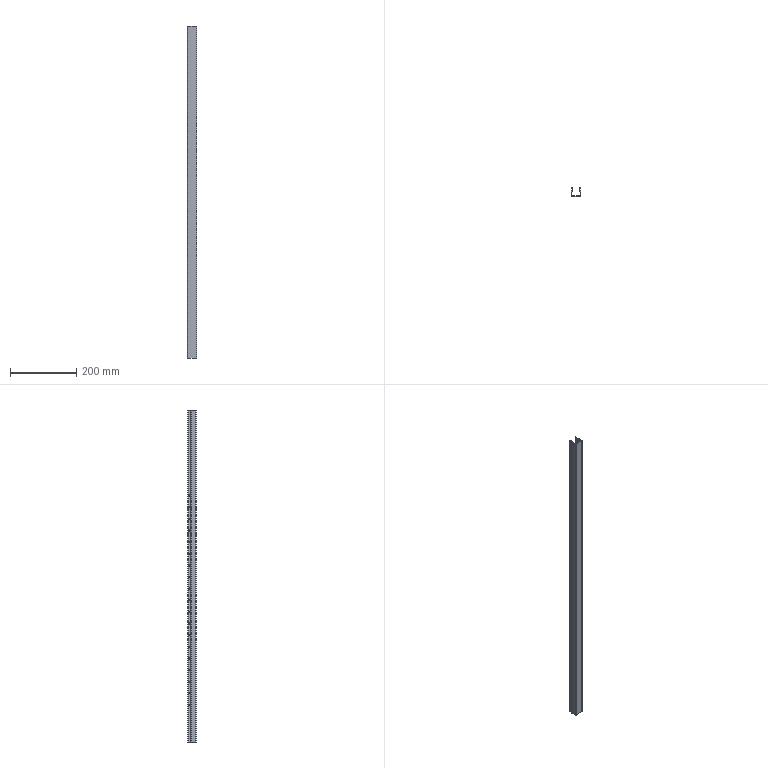Part | STEP file | GALVANIZED RAIL 02 | 1 solid | 120 faces | box 28.4 x 26.2 x 999 mm | volume 99426 mm3 | cylinder 92 | plane 28 | commonest cylinder face diameters 4 x76 1.473 x8 3.873 x8